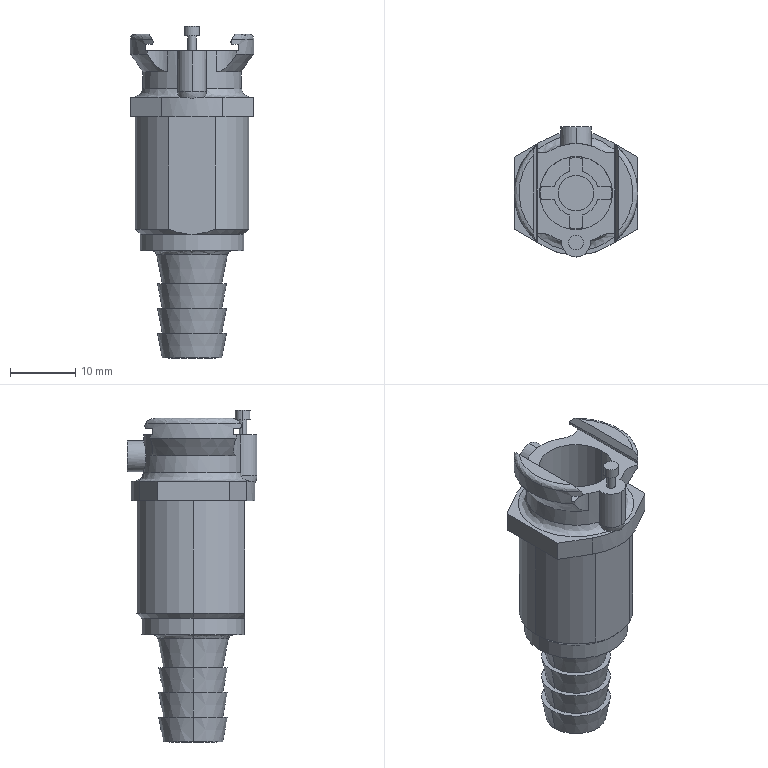Part | SolidWorks | features BaseBody 1 | 1 solid | 102 faces | box 19.05 x 19.99 x 51.054 mm | volume 5563 mm3 | cylinder 42 | plane 40 | cone 13 | spline 7 | commonest cylinder face diameters 10.871 x5 6.096 x4 7.01 x4 11.252 x4 19.05 x4 17.462 x3